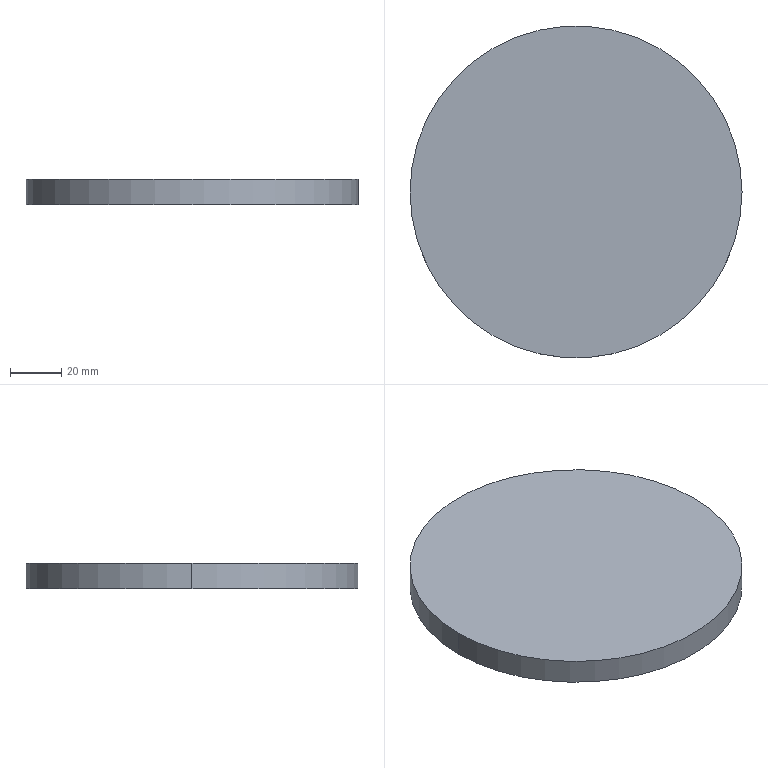Part | SolidWorks | features Extrusion 1 | 1 solid | 4 faces | box 130 x 130 x 10 mm | volume 132732 mm3 | cylinder 2 | plane 2 | commonest cylinder face diameters 130 x2
STEP:
#1=CARTESIAN_POINT('',(65.,0.,10.));
#2=VERTEX_POINT('',#1);
#3=CARTESIAN_POINT('',(-65.,0.,10.));
#4=VERTEX_POINT('',#3);
#5=CARTESIAN_POINT('',(0.,0.,10.));
#6=DIRECTION('',(0.,0.,1.));
#7=DIRECTION('',(1.,0.,0.));
#8=AXIS2_PLACEMENT_3D('',#5,#6,#7);
#9=CIRCLE('',#8,65.);
#10=EDGE_CURVE('',#2,#4,#9,.T.);
#11=ORIENTED_EDGE('',*,*,#10,.F.);
#12=CARTESIAN_POINT('',(65.,0.,0.));
#13=VERTEX_POINT('',#12);
#14=CARTESIAN_POINT('',(65.,0.,10.));
#15=DIRECTION('',(0.,0.,-1.));
#16=VECTOR('',#15,1000.);
#17=LINE('',#14,#16);
#18=EDGE_CURVE('',#2,#13,#17,.T.);
#19=ORIENTED_EDGE('',*,*,#18,.T.);
#20=CARTESIAN_POINT('',(-65.,0.,0.));
#21=VERTEX_POINT('',#20);
#22=CARTESIAN_POINT('',(0.,0.,0.));
#23=DIRECTION('',(0.,0.,1.));
#24=DIRECTION('',(1.,0.,0.));
#25=AXIS2_PLACEMENT_3D('',#22,#23,#24);
#26=CIRCLE('',#25,65.);
#27=EDGE_CURVE('',#13,#21,#26,.T.);
#28=ORIENTED_EDGE('',*,*,#27,.T.);
#29=CARTESIAN_POINT('',(-65.,0.,10.));
#30=DIRECTION('',(0.,0.,-1.));
#31=VECTOR('',#30,1000.);
#32=LINE('',#29,#31);
#33=EDGE_CURVE('',#4,#21,#32,.T.);
#34=ORIENTED_EDGE('',*,*,#33,.F.);
#35=EDGE_LOOP('',(#11,#19,#28,#34));
#36=FACE_OUTER_BOUND('',#35,.T.);
#37=CARTESIAN_POINT('',(0.,0.,10.));
#38=DIRECTION('',(0.,0.,-1.));
#39=DIRECTION('',(-1.,0.,0.));
#40=AXIS2_PLACEMENT_3D('',#37,#38,#39);
#41=CYLINDRICAL_SURFACE('',#40,65.);
#42=ADVANCED_FACE('',(#36),#41,.T.);
#43=ORIENTED_EDGE('',*,*,#18,.F.);
#44=CARTESIAN_POINT('',(0.,0.,10.));
#45=DIRECTION('',(0.,0.,1.));
#46=DIRECTION('',(1.,0.,0.));
#47=AXIS2_PLACEMENT_3D('',#44,#45,#46);
#48=CIRCLE('',#47,65.);
#49=EDGE_CURVE('',#4,#2,#48,.T.);
#50=ORIENTED_EDGE('',*,*,#49,.F.);
#51=ORIENTED_EDGE('',*,*,#33,.T.);
#52=CARTESIAN_POINT('',(0.,0.,0.));
#53=DIRECTION('',(0.,0.,1.));
#54=DIRECTION('',(1.,0.,0.));
#55=AXIS2_PLACEMENT_3D('',#52,#53,#54);
#56=CIRCLE('',#55,65.);
#57=EDGE_CURVE('',#21,#13,#56,.T.);
#58=ORIENTED_EDGE('',*,*,#57,.T.);
#59=EDGE_LOOP('',(#43,#50,#51,#58));
#60=FACE_OUTER_BOUND('',#59,.T.);
#61=CARTESIAN_POINT('',(0.,0.,10.));
#62=DIRECTION('',(0.,0.,-1.));
#63=DIRECTION('',(-1.,0.,0.));
#64=AXIS2_PLACEMENT_3D('',#61,#62,#63);
#65=CYLINDRICAL_SURFACE('',#64,65.);
#66=ADVANCED_FACE('',(#60),#65,.T.);
#67=ORIENTED_EDGE('',*,*,#49,.T.);
#68=ORIENTED_EDGE('',*,*,#10,.T.);
#69=EDGE_LOOP('',(#67,#68));
#70=FACE_OUTER_BOUND('',#69,.T.);
#71=CARTESIAN_POINT('',(0.,0.,10.));
#72=DIRECTION('',(0.,0.,1.));
#73=DIRECTION('',(1.,0.,0.));
#74=AXIS2_PLACEMENT_3D('',#71,#72,#73);
#75=PLANE('',#74);
#76=ADVANCED_FACE('',(#70),#75,.T.);
#77=ORIENTED_EDGE('',*,*,#57,.F.);
#78=ORIENTED_EDGE('',*,*,#27,.F.);
#79=EDGE_LOOP('',(#77,#78));
#80=FACE_OUTER_BOUND('',#79,.T.);
#81=CARTESIAN_POINT('',(0.,0.,0.));
#82=DIRECTION('',(0.,0.,1.));
#83=DIRECTION('',(1.,0.,0.));
#84=AXIS2_PLACEMENT_3D('',#81,#82,#83);
#85=PLANE('',#84);
#86=ADVANCED_FACE('',(#80),#85,.F.);
#87=CLOSED_SHELL('',(#42,#66,#76,#86));
#88=MANIFOLD_SOLID_BREP('',#87);
#89=CARTESIAN_POINT('',(0.,0.,0.));
#90=DIRECTION('',(0.,0.,1.));
#91=DIRECTION('',(1.,0.,0.));
#92=AXIS2_PLACEMENT_3D('',#89,#90,#91);
#93=(LENGTH_UNIT()NAMED_UNIT(*)SI_UNIT(.MILLI.,.METRE.));
#94=UNCERTAINTY_MEASURE_WITH_UNIT(LENGTH_MEASURE(0.00001),#93,'','');
#95=(NAMED_UNIT(*)PLANE_ANGLE_UNIT()SI_UNIT($,.RADIAN.));
#96=(NAMED_UNIT(*)SI_UNIT($,.STERADIAN.)SOLID_ANGLE_UNIT());
#97=(GEOMETRIC_REPRESENTATION_CONTEXT(3)GLOBAL_UNCERTAINTY_ASSIGNED_CONTEXT((#94))GLOBAL_UNIT_ASSIGNED_CONTEXT((#93,#95,#96))REPRESENTATION_CONTEXT('',''));
#98=ADVANCED_BREP_SHAPE_REPRESENTATION('',(#88,#92),#97);